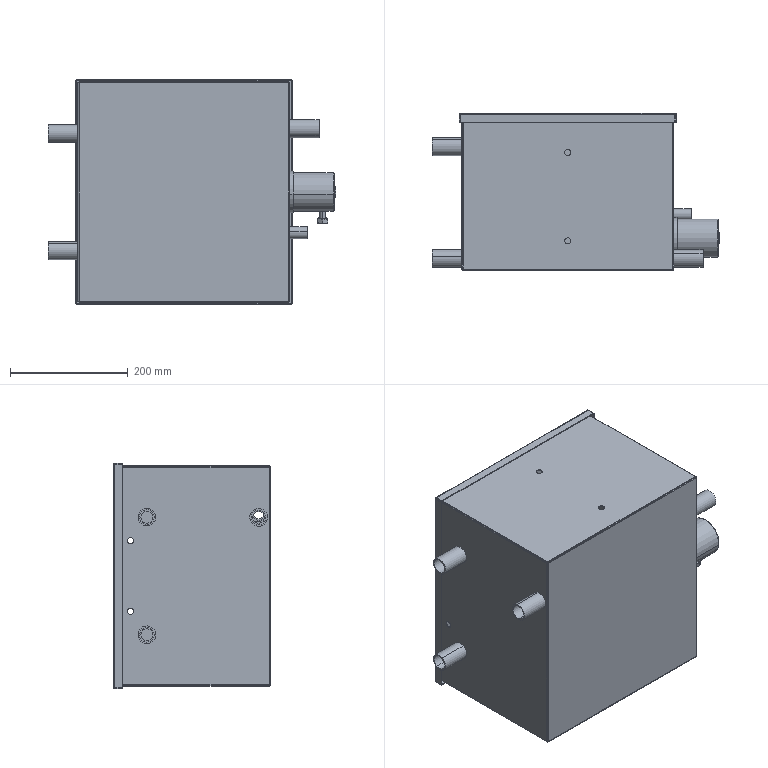Part | SolidWorks | features CompositeCurve 7 | 8 solids | 211 faces | box 488 x 266.5 x 384 mm | volume 1398529 mm3 | cylinder 92 | plane 85 | spline 24 | torus 6 | cone 4 | commonest cylinder face diameters 1 x12 4 x12 10.5 x12 20 x12 5 x8 25 x8